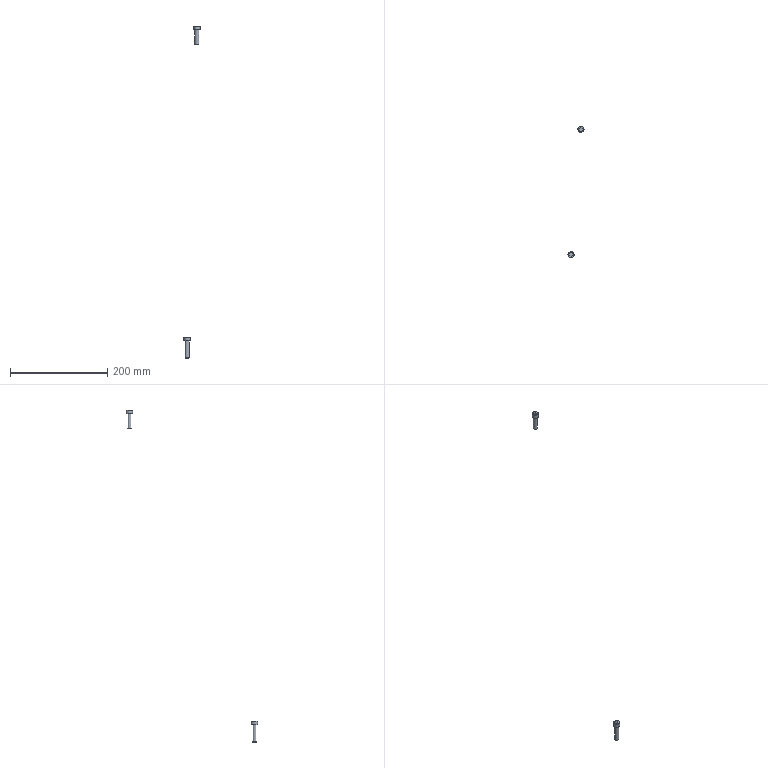Part | STEP file | M8.00-35 | 2 solids | 28 faces | box 33.038 x 270 x 682.52 mm | volume 5048 mm3 | plane 20 | cylinder 4 | cone 4 | commonest cylinder face diameters 8 x2 13 x2